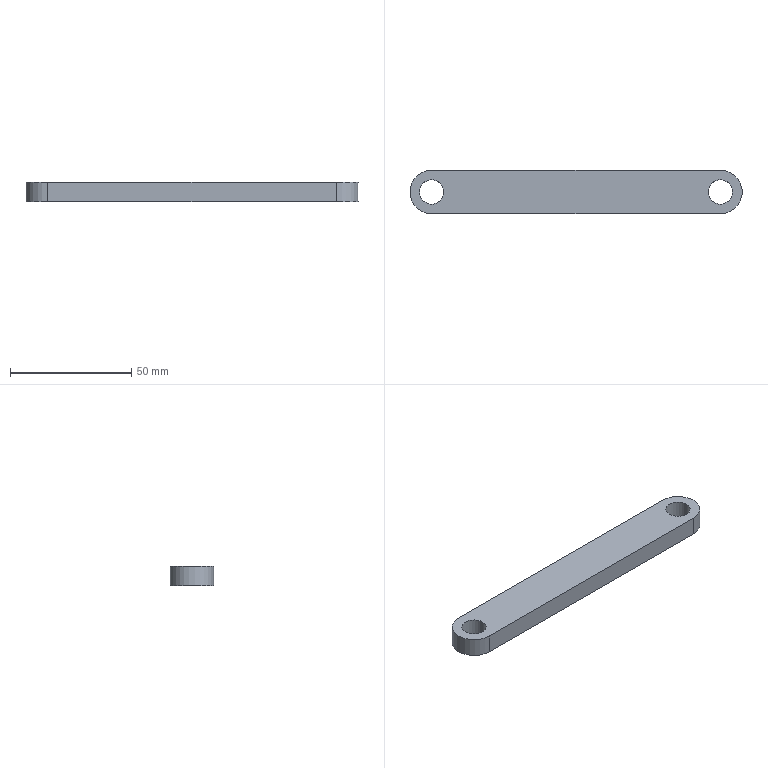Part | STEP file | Crank | 1 solid | 8 faces | box 136.8 x 18 x 8 mm | volume 17886 mm3 | plane 4 | cylinder 4 | commonest cylinder face diameters 10 x2 18 x2
STEP:
#1=CARTESIAN_POINT('',(0.,0.,0.));
#2=DIRECTION('',(0.,0.,1.));
#3=DIRECTION('',(1.,0.,0.));
#4=AXIS2_PLACEMENT_3D('',#1,#2,#3);
#5=CARTESIAN_POINT('',(123.8,0.,8.));
#6=VERTEX_POINT('',#5);
#7=CARTESIAN_POINT('',(118.8,0.,8.));
#8=DIRECTION('',(0.,0.,1.));
#9=DIRECTION('',(1.,0.,0.));
#10=AXIS2_PLACEMENT_3D('',#7,#8,#9);
#11=CIRCLE('',#10,5.);
#12=CARTESIAN_POINT('',(0.,0.,8.));
#13=DIRECTION('',(0.,0.,1.));
#14=DIRECTION('',(1.,0.,0.));
#15=AXIS2_PLACEMENT_3D('',#12,#13,#14);
#16=PLANE('',#15);
#17=CARTESIAN_POINT('',(118.8,0.));
#18=DIRECTION('',(1.,0.));
#19=AXIS2_PLACEMENT_2D('',#17,#18);
#20=CIRCLE('',#19,5.);
#21=(GEOMETRIC_REPRESENTATION_CONTEXT(2)PARAMETRIC_REPRESENTATION_CONTEXT()REPRESENTATION_CONTEXT('',''));
#22=DEFINITIONAL_REPRESENTATION('',(#20),#21);
#23=PCURVE('',#16,#22);
#24=CARTESIAN_POINT('',(118.8,0.,8.));
#25=DIRECTION('',(0.,0.,-1.));
#26=DIRECTION('',(-1.,0.,0.));
#27=AXIS2_PLACEMENT_3D('',#24,#25,#26);
#28=CYLINDRICAL_SURFACE('',#27,5.);
#29=CARTESIAN_POINT('',(9.425,0.));
#30=DIRECTION('',(-1.,0.));
#31=VECTOR('',#30,1.);
#32=LINE('',#29,#31);
#33=(GEOMETRIC_REPRESENTATION_CONTEXT(2)PARAMETRIC_REPRESENTATION_CONTEXT()REPRESENTATION_CONTEXT('',''));
#34=DEFINITIONAL_REPRESENTATION('',(#32),#33);
#35=PCURVE('',#28,#34);
#36=SURFACE_CURVE('',#11,(#23,#35),.PCURVE_S1.);
#37=EDGE_CURVE('',#6,#6,#36,.T.);
#38=ORIENTED_EDGE('',*,*,#37,.F.);
#39=EDGE_LOOP('',(#38));
#40=FACE_BOUND('',#39,.T.);
#41=CARTESIAN_POINT('',(0.,9.,8.));
#42=VERTEX_POINT('',#41);
#43=CARTESIAN_POINT('',(0.,-9.,8.));
#44=VERTEX_POINT('',#43);
#45=CARTESIAN_POINT('',(0.,0.,8.));
#46=DIRECTION('',(0.,0.,1.));
#47=DIRECTION('',(1.,0.,0.));
#48=AXIS2_PLACEMENT_3D('',#45,#46,#47);
#49=CIRCLE('',#48,9.);
#50=CARTESIAN_POINT('',(0.,0.));
#51=DIRECTION('',(1.,0.));
#52=AXIS2_PLACEMENT_2D('',#50,#51);
#53=CIRCLE('',#52,9.);
#54=(GEOMETRIC_REPRESENTATION_CONTEXT(2)PARAMETRIC_REPRESENTATION_CONTEXT()REPRESENTATION_CONTEXT('',''));
#55=DEFINITIONAL_REPRESENTATION('',(#53),#54);
#56=PCURVE('',#16,#55);
#57=CARTESIAN_POINT('',(0.,0.,8.));
#58=DIRECTION('',(0.,0.,-1.));
#59=DIRECTION('',(-1.,0.,0.));
#60=AXIS2_PLACEMENT_3D('',#57,#58,#59);
#61=CYLINDRICAL_SURFACE('',#60,9.);
#62=CARTESIAN_POINT('',(3.142,0.));
#63=DIRECTION('',(-1.,0.));
#64=VECTOR('',#63,1.);
#65=LINE('',#62,#64);
#66=(GEOMETRIC_REPRESENTATION_CONTEXT(2)PARAMETRIC_REPRESENTATION_CONTEXT()REPRESENTATION_CONTEXT('',''));
#67=DEFINITIONAL_REPRESENTATION('',(#65),#66);
#68=PCURVE('',#61,#67);
#69=SURFACE_CURVE('',#49,(#56,#68),.PCURVE_S1.);
#70=EDGE_CURVE('',#42,#44,#69,.T.);
#71=ORIENTED_EDGE('',*,*,#70,.T.);
#72=CARTESIAN_POINT('',(118.8,-9.,8.));
#73=VERTEX_POINT('',#72);
#74=CARTESIAN_POINT('',(0.,-9.,8.));
#75=DIRECTION('',(1.,0.,0.));
#76=VECTOR('',#75,1.);
#77=LINE('',#74,#76);
#78=CARTESIAN_POINT('',(0.,-9.));
#79=DIRECTION('',(1.,0.));
#80=VECTOR('',#79,1.);
#81=LINE('',#78,#80);
#82=(GEOMETRIC_REPRESENTATION_CONTEXT(2)PARAMETRIC_REPRESENTATION_CONTEXT()REPRESENTATION_CONTEXT('',''));
#83=DEFINITIONAL_REPRESENTATION('',(#81),#82);
#84=PCURVE('',#16,#83);
#85=CARTESIAN_POINT('',(0.,-9.,8.));
#86=DIRECTION('',(0.,1.,0.));
#87=DIRECTION('',(0.,0.,1.));
#88=AXIS2_PLACEMENT_3D('',#85,#86,#87);
#89=PLANE('',#88);
#90=CARTESIAN_POINT('',(0.,0.));
#91=DIRECTION('',(0.,1.));
#92=VECTOR('',#91,1.);
#93=LINE('',#90,#92);
#94=(GEOMETRIC_REPRESENTATION_CONTEXT(2)PARAMETRIC_REPRESENTATION_CONTEXT()REPRESENTATION_CONTEXT('',''));
#95=DEFINITIONAL_REPRESENTATION('',(#93),#94);
#96=PCURVE('',#89,#95);
#97=SURFACE_CURVE('',#77,(#84,#96),.PCURVE_S1.);
#98=EDGE_CURVE('',#44,#73,#97,.T.);
#99=ORIENTED_EDGE('',*,*,#98,.T.);
#100=CARTESIAN_POINT('',(118.8,9.,8.));
#101=VERTEX_POINT('',#100);
#102=CARTESIAN_POINT('',(118.8,0.,8.));
#103=DIRECTION('',(0.,0.,1.));
#104=DIRECTION('',(1.,0.,0.));
#105=AXIS2_PLACEMENT_3D('',#102,#103,#104);
#106=CIRCLE('',#105,9.);
#107=CARTESIAN_POINT('',(118.8,0.));
#108=DIRECTION('',(1.,0.));
#109=AXIS2_PLACEMENT_2D('',#107,#108);
#110=CIRCLE('',#109,9.);
#111=(GEOMETRIC_REPRESENTATION_CONTEXT(2)PARAMETRIC_REPRESENTATION_CONTEXT()REPRESENTATION_CONTEXT('',''));
#112=DEFINITIONAL_REPRESENTATION('',(#110),#111);
#113=PCURVE('',#16,#112);
#114=CARTESIAN_POINT('',(118.8,0.,8.));
#115=DIRECTION('',(0.,0.,-1.));
#116=DIRECTION('',(-1.,0.,0.));
#117=AXIS2_PLACEMENT_3D('',#114,#115,#116);
#118=CYLINDRICAL_SURFACE('',#117,9.);
#119=CARTESIAN_POINT('',(9.425,0.));
#120=DIRECTION('',(-1.,0.));
#121=VECTOR('',#120,1.);
#122=LINE('',#119,#121);
#123=(GEOMETRIC_REPRESENTATION_CONTEXT(2)PARAMETRIC_REPRESENTATION_CONTEXT()REPRESENTATION_CONTEXT('',''));
#124=DEFINITIONAL_REPRESENTATION('',(#122),#123);
#125=PCURVE('',#118,#124);
#126=SURFACE_CURVE('',#106,(#113,#125),.PCURVE_S1.);
#127=EDGE_CURVE('',#73,#101,#126,.T.);
#128=ORIENTED_EDGE('',*,*,#127,.T.);
#129=CARTESIAN_POINT('',(0.,9.,8.));
#130=DIRECTION('',(-1.,0.,0.));
#131=VECTOR('',#130,1.);
#132=LINE('',#129,#131);
#133=CARTESIAN_POINT('',(0.,9.));
#134=DIRECTION('',(-1.,0.));
#135=VECTOR('',#134,1.);
#136=LINE('',#133,#135);
#137=(GEOMETRIC_REPRESENTATION_CONTEXT(2)PARAMETRIC_REPRESENTATION_CONTEXT()REPRESENTATION_CONTEXT('',''));
#138=DEFINITIONAL_REPRESENTATION('',(#136),#137);
#139=PCURVE('',#16,#138);
#140=CARTESIAN_POINT('',(0.,9.,8.));
#141=DIRECTION('',(0.,-1.,0.));
#142=DIRECTION('',(0.,0.,-1.));
#143=AXIS2_PLACEMENT_3D('',#140,#141,#142);
#144=PLANE('',#143);
#145=CARTESIAN_POINT('',(0.,0.));
#146=DIRECTION('',(0.,-1.));
#147=VECTOR('',#146,1.);
#148=LINE('',#145,#147);
#149=(GEOMETRIC_REPRESENTATION_CONTEXT(2)PARAMETRIC_REPRESENTATION_CONTEXT()REPRESENTATION_CONTEXT('',''));
#150=DEFINITIONAL_REPRESENTATION('',(#148),#149);
#151=PCURVE('',#144,#150);
#152=SURFACE_CURVE('',#132,(#139,#151),.PCURVE_S1.);
#153=EDGE_CURVE('',#101,#42,#152,.T.);
#154=ORIENTED_EDGE('',*,*,#153,.T.);
#155=EDGE_LOOP('',(#71,#99,#128,#154));
#156=FACE_BOUND('',#155,.T.);
#157=CARTESIAN_POINT('',(5.,0.,8.));
#158=VERTEX_POINT('',#157);
#159=CARTESIAN_POINT('',(0.,0.,8.));
#160=DIRECTION('',(0.,0.,1.));
#161=DIRECTION('',(1.,0.,0.));
#162=AXIS2_PLACEMENT_3D('',#159,#160,#161);
#163=CIRCLE('',#162,5.);
#164=CARTESIAN_POINT('',(0.,0.));
#165=DIRECTION('',(1.,0.));
#166=AXIS2_PLACEMENT_2D('',#164,#165);
#167=CIRCLE('',#166,5.);
#168=(GEOMETRIC_REPRESENTATION_CONTEXT(2)PARAMETRIC_REPRESENTATION_CONTEXT()REPRESENTATION_CONTEXT('',''));
#169=DEFINITIONAL_REPRESENTATION('',(#167),#168);
#170=PCURVE('',#16,#169);
#171=CARTESIAN_POINT('',(0.,0.,8.));
#172=DIRECTION('',(0.,0.,-1.));
#173=DIRECTION('',(-1.,0.,0.));
#174=AXIS2_PLACEMENT_3D('',#171,#172,#173);
#175=CYLINDRICAL_SURFACE('',#174,5.);
#176=CARTESIAN_POINT('',(9.425,0.));
#177=DIRECTION('',(-1.,0.));
#178=VECTOR('',#177,1.);
#179=LINE('',#176,#178);
#180=(GEOMETRIC_REPRESENTATION_CONTEXT(2)PARAMETRIC_REPRESENTATION_CONTEXT()REPRESENTATION_CONTEXT('',''));
#181=DEFINITIONAL_REPRESENTATION('',(#179),#180);
#182=PCURVE('',#175,#181);
#183=SURFACE_CURVE('',#163,(#170,#182),.PCURVE_S1.);
#184=EDGE_CURVE('',#158,#158,#183,.T.);
#185=ORIENTED_EDGE('',*,*,#184,.F.);
#186=EDGE_LOOP('',(#185));
#187=FACE_BOUND('',#186,.T.);
#188=ADVANCED_FACE('',(#40,#156,#187),#16,.T.);
#189=CARTESIAN_POINT('',(0.,9.,0.));
#190=VERTEX_POINT('',#189);
#191=CARTESIAN_POINT('',(0.,-9.,0.));
#192=VERTEX_POINT('',#191);
#193=CARTESIAN_POINT('',(0.,0.,0.));
#194=DIRECTION('',(0.,0.,1.));
#195=DIRECTION('',(1.,0.,0.));
#196=AXIS2_PLACEMENT_3D('',#193,#194,#195);
#197=CIRCLE('',#196,9.);
#198=CARTESIAN_POINT('',(0.,0.,0.));
#199=DIRECTION('',(0.,0.,1.));
#200=DIRECTION('',(1.,0.,0.));
#201=AXIS2_PLACEMENT_3D('',#198,#199,#200);
#202=PLANE('',#201);
#203=CARTESIAN_POINT('',(0.,0.));
#204=DIRECTION('',(1.,0.));
#205=AXIS2_PLACEMENT_2D('',#203,#204);
#206=CIRCLE('',#205,9.);
#207=(GEOMETRIC_REPRESENTATION_CONTEXT(2)PARAMETRIC_REPRESENTATION_CONTEXT()REPRESENTATION_CONTEXT('',''));
#208=DEFINITIONAL_REPRESENTATION('',(#206),#207);
#209=PCURVE('',#202,#208);
#210=CARTESIAN_POINT('',(3.142,8.));
#211=DIRECTION('',(-1.,0.));
#212=VECTOR('',#211,1.);
#213=LINE('',#210,#212);
#214=(GEOMETRIC_REPRESENTATION_CONTEXT(2)PARAMETRIC_REPRESENTATION_CONTEXT()REPRESENTATION_CONTEXT('',''));
#215=DEFINITIONAL_REPRESENTATION('',(#213),#214);
#216=PCURVE('',#61,#215);
#217=SURFACE_CURVE('',#197,(#209,#216),.PCURVE_S1.);
#218=EDGE_CURVE('',#190,#192,#217,.T.);
#219=ORIENTED_EDGE('',*,*,#218,.F.);
#220=CARTESIAN_POINT('',(118.8,9.,0.));
#221=VERTEX_POINT('',#220);
#222=CARTESIAN_POINT('',(0.,9.,0.));
#223=DIRECTION('',(-1.,0.,0.));
#224=VECTOR('',#223,1.);
#225=LINE('',#222,#224);
#226=CARTESIAN_POINT('',(0.,9.));
#227=DIRECTION('',(-1.,0.));
#228=VECTOR('',#227,1.);
#229=LINE('',#226,#228);
#230=(GEOMETRIC_REPRESENTATION_CONTEXT(2)PARAMETRIC_REPRESENTATION_CONTEXT()REPRESENTATION_CONTEXT('',''));
#231=DEFINITIONAL_REPRESENTATION('',(#229),#230);
#232=PCURVE('',#202,#231);
#233=CARTESIAN_POINT('',(8.,0.));
#234=DIRECTION('',(0.,-1.));
#235=VECTOR('',#234,1.);
#236=LINE('',#233,#235);
#237=(GEOMETRIC_REPRESENTATION_CONTEXT(2)PARAMETRIC_REPRESENTATION_CONTEXT()REPRESENTATION_CONTEXT('',''));
#238=DEFINITIONAL_REPRESENTATION('',(#236),#237);
#239=PCURVE('',#144,#238);
#240=SURFACE_CURVE('',#225,(#232,#239),.PCURVE_S1.);
#241=EDGE_CURVE('',#221,#190,#240,.T.);
#242=ORIENTED_EDGE('',*,*,#241,.F.);
#243=CARTESIAN_POINT('',(118.8,-9.,0.));
#244=VERTEX_POINT('',#243);
#245=CARTESIAN_POINT('',(118.8,0.,0.));
#246=DIRECTION('',(0.,0.,1.));
#247=DIRECTION('',(1.,0.,0.));
#248=AXIS2_PLACEMENT_3D('',#245,#246,#247);
#249=CIRCLE('',#248,9.);
#250=CARTESIAN_POINT('',(118.8,0.));
#251=DIRECTION('',(1.,0.));
#252=AXIS2_PLACEMENT_2D('',#250,#251);
#253=CIRCLE('',#252,9.);
#254=(GEOMETRIC_REPRESENTATION_CONTEXT(2)PARAMETRIC_REPRESENTATION_CONTEXT()REPRESENTATION_CONTEXT('',''));
#255=DEFINITIONAL_REPRESENTATION('',(#253),#254);
#256=PCURVE('',#202,#255);
#257=CARTESIAN_POINT('',(9.425,8.));
#258=DIRECTION('',(-1.,0.));
#259=VECTOR('',#258,1.);
#260=LINE('',#257,#259);
#261=(GEOMETRIC_REPRESENTATION_CONTEXT(2)PARAMETRIC_REPRESENTATION_CONTEXT()REPRESENTATION_CONTEXT('',''));
#262=DEFINITIONAL_REPRESENTATION('',(#260),#261);
#263=PCURVE('',#118,#262);
#264=SURFACE_CURVE('',#249,(#256,#263),.PCURVE_S1.);
#265=EDGE_CURVE('',#244,#221,#264,.T.);
#266=ORIENTED_EDGE('',*,*,#265,.F.);
#267=CARTESIAN_POINT('',(0.,-9.,0.));
#268=DIRECTION('',(1.,0.,0.));
#269=VECTOR('',#268,1.);
#270=LINE('',#267,#269);
#271=CARTESIAN_POINT('',(0.,-9.));
#272=DIRECTION('',(1.,0.));
#273=VECTOR('',#272,1.);
#274=LINE('',#271,#273);
#275=(GEOMETRIC_REPRESENTATION_CONTEXT(2)PARAMETRIC_REPRESENTATION_CONTEXT()REPRESENTATION_CONTEXT('',''));
#276=DEFINITIONAL_REPRESENTATION('',(#274),#275);
#277=PCURVE('',#202,#276);
#278=CARTESIAN_POINT('',(-8.,0.));
#279=DIRECTION('',(0.,1.));
#280=VECTOR('',#279,1.);
#281=LINE('',#278,#280);
#282=(GEOMETRIC_REPRESENTATION_CONTEXT(2)PARAMETRIC_REPRESENTATION_CONTEXT()REPRESENTATION_CONTEXT('',''));
#283=DEFINITIONAL_REPRESENTATION('',(#281),#282);
#284=PCURVE('',#89,#283);
#285=SURFACE_CURVE('',#270,(#277,#284),.PCURVE_S1.);
#286=EDGE_CURVE('',#192,#244,#285,.T.);
#287=ORIENTED_EDGE('',*,*,#286,.F.);
#288=EDGE_LOOP('',(#219,#242,#266,#287));
#289=FACE_BOUND('',#288,.T.);
#290=CARTESIAN_POINT('',(123.8,0.,0.));
#291=VERTEX_POINT('',#290);
#292=CARTESIAN_POINT('',(118.8,0.,0.));
#293=DIRECTION('',(0.,0.,1.));
#294=DIRECTION('',(1.,0.,0.));
#295=AXIS2_PLACEMENT_3D('',#292,#293,#294);
#296=CIRCLE('',#295,5.);
#297=CARTESIAN_POINT('',(118.8,0.));
#298=DIRECTION('',(1.,0.));
#299=AXIS2_PLACEMENT_2D('',#297,#298);
#300=CIRCLE('',#299,5.);
#301=(GEOMETRIC_REPRESENTATION_CONTEXT(2)PARAMETRIC_REPRESENTATION_CONTEXT()REPRESENTATION_CONTEXT('',''));
#302=DEFINITIONAL_REPRESENTATION('',(#300),#301);
#303=PCURVE('',#202,#302);
#304=CARTESIAN_POINT('',(9.425,8.));
#305=DIRECTION('',(-1.,0.));
#306=VECTOR('',#305,1.);
#307=LINE('',#304,#306);
#308=(GEOMETRIC_REPRESENTATION_CONTEXT(2)PARAMETRIC_REPRESENTATION_CONTEXT()REPRESENTATION_CONTEXT('',''));
#309=DEFINITIONAL_REPRESENTATION('',(#307),#308);
#310=PCURVE('',#28,#309);
#311=SURFACE_CURVE('',#296,(#303,#310),.PCURVE_S1.);
#312=EDGE_CURVE('',#291,#291,#311,.T.);
#313=ORIENTED_EDGE('',*,*,#312,.T.);
#314=EDGE_LOOP('',(#313));
#315=FACE_BOUND('',#314,.T.);
#316=CARTESIAN_POINT('',(5.,0.,0.));
#317=VERTEX_POINT('',#316);
#318=CARTESIAN_POINT('',(0.,0.,0.));
#319=DIRECTION('',(0.,0.,1.));
#320=DIRECTION('',(1.,0.,0.));
#321=AXIS2_PLACEMENT_3D('',#318,#319,#320);
#322=CIRCLE('',#321,5.);
#323=CARTESIAN_POINT('',(0.,0.));
#324=DIRECTION('',(1.,0.));
#325=AXIS2_PLACEMENT_2D('',#323,#324);
#326=CIRCLE('',#325,5.);
#327=(GEOMETRIC_REPRESENTATION_CONTEXT(2)PARAMETRIC_REPRESENTATION_CONTEXT()REPRESENTATION_CONTEXT('',''));
#328=DEFINITIONAL_REPRESENTATION('',(#326),#327);
#329=PCURVE('',#202,#328);
#330=CARTESIAN_POINT('',(9.425,8.));
#331=DIRECTION('',(-1.,0.));
#332=VECTOR('',#331,1.);
#333=LINE('',#330,#332);
#334=(GEOMETRIC_REPRESENTATION_CONTEXT(2)PARAMETRIC_REPRESENTATION_CONTEXT()REPRESENTATION_CONTEXT('',''));
#335=DEFINITIONAL_REPRESENTATION('',(#333),#334);
#336=PCURVE('',#175,#335);
#337=SURFACE_CURVE('',#322,(#329,#336),.PCURVE_S1.);
#338=EDGE_CURVE('',#317,#317,#337,.T.);
#339=ORIENTED_EDGE('',*,*,#338,.T.);
#340=EDGE_LOOP('',(#339));
#341=FACE_BOUND('',#340,.T.);
#342=ADVANCED_FACE('',(#289,#315,#341),#202,.F.);
#343=ORIENTED_EDGE('',*,*,#218,.T.);
#344=CARTESIAN_POINT('',(0.,-9.,8.));
#345=DIRECTION('',(0.,0.,-1.));
#346=VECTOR('',#345,1.);
#347=LINE('',#344,#346);
#348=CARTESIAN_POINT('',(-1.571,0.));
#349=DIRECTION('',(0.,1.));
#350=VECTOR('',#349,1.);
#351=LINE('',#348,#350);
#352=(GEOMETRIC_REPRESENTATION_CONTEXT(2)PARAMETRIC_REPRESENTATION_CONTEXT()REPRESENTATION_CONTEXT('',''));
#353=DEFINITIONAL_REPRESENTATION('',(#351),#352);
#354=PCURVE('',#61,#353);
#355=CARTESIAN_POINT('',(0.,0.));
#356=DIRECTION('',(-1.,0.));
#357=VECTOR('',#356,1.);
#358=LINE('',#355,#357);
#359=(GEOMETRIC_REPRESENTATION_CONTEXT(2)PARAMETRIC_REPRESENTATION_CONTEXT()REPRESENTATION_CONTEXT('',''));
#360=DEFINITIONAL_REPRESENTATION('',(#358),#359);
#361=PCURVE('',#89,#360);
#362=SURFACE_CURVE('',#347,(#354,#361),.PCURVE_S1.);
#363=EDGE_CURVE('',#44,#192,#362,.T.);
#364=ORIENTED_EDGE('',*,*,#363,.F.);
#365=ORIENTED_EDGE('',*,*,#70,.F.);
#366=CARTESIAN_POINT('',(0.,9.,8.));
#367=DIRECTION('',(0.,0.,-1.));
#368=VECTOR('',#367,1.);
#369=LINE('',#366,#368);
#370=CARTESIAN_POINT('',(1.571,0.));
#371=DIRECTION('',(0.,1.));
#372=VECTOR('',#371,1.);
#373=LINE('',#370,#372);
#374=(GEOMETRIC_REPRESENTATION_CONTEXT(2)PARAMETRIC_REPRESENTATION_CONTEXT()REPRESENTATION_CONTEXT('',''));
#375=DEFINITIONAL_REPRESENTATION('',(#373),#374);
#376=PCURVE('',#61,#375);
#377=CARTESIAN_POINT('',(0.,0.));
#378=DIRECTION('',(1.,0.));
#379=VECTOR('',#378,1.);
#380=LINE('',#377,#379);
#381=(GEOMETRIC_REPRESENTATION_CONTEXT(2)PARAMETRIC_REPRESENTATION_CONTEXT()REPRESENTATION_CONTEXT('',''));
#382=DEFINITIONAL_REPRESENTATION('',(#380),#381);
#383=PCURVE('',#144,#382);
#384=SURFACE_CURVE('',#369,(#376,#383),.PCURVE_S1.);
#385=EDGE_CURVE('',#42,#190,#384,.T.);
#386=ORIENTED_EDGE('',*,*,#385,.T.);
#387=EDGE_LOOP('',(#343,#364,#365,#386));
#388=FACE_BOUND('',#387,.T.);
#389=ADVANCED_FACE('',(#388),#61,.T.);
#390=ORIENTED_EDGE('',*,*,#286,.T.);
#391=CARTESIAN_POINT('',(118.8,-9.,8.));
#392=DIRECTION('',(0.,0.,-1.));
#393=VECTOR('',#392,1.);
#394=LINE('',#391,#393);
#395=CARTESIAN_POINT('',(0.,118.8));
#396=DIRECTION('',(-1.,0.));
#397=VECTOR('',#396,1.);
#398=LINE('',#395,#397);
#399=(GEOMETRIC_REPRESENTATION_CONTEXT(2)PARAMETRIC_REPRESENTATION_CONTEXT()REPRESENTATION_CONTEXT('',''));
#400=DEFINITIONAL_REPRESENTATION('',(#398),#399);
#401=PCURVE('',#89,#400);
#402=CARTESIAN_POINT('',(4.712,0.));
#403=DIRECTION('',(0.,1.));
#404=VECTOR('',#403,1.);
#405=LINE('',#402,#404);
#406=(GEOMETRIC_REPRESENTATION_CONTEXT(2)PARAMETRIC_REPRESENTATION_CONTEXT()REPRESENTATION_CONTEXT('',''));
#407=DEFINITIONAL_REPRESENTATION('',(#405),#406);
#408=PCURVE('',#118,#407);
#409=SURFACE_CURVE('',#394,(#401,#408),.PCURVE_S1.);
#410=EDGE_CURVE('',#73,#244,#409,.T.);
#411=ORIENTED_EDGE('',*,*,#410,.F.);
#412=ORIENTED_EDGE('',*,*,#98,.F.);
#413=ORIENTED_EDGE('',*,*,#363,.T.);
#414=EDGE_LOOP('',(#390,#411,#412,#413));
#415=FACE_BOUND('',#414,.T.);
#416=ADVANCED_FACE('',(#415),#89,.F.);
#417=ORIENTED_EDGE('',*,*,#265,.T.);
#418=CARTESIAN_POINT('',(118.8,9.,8.));
#419=DIRECTION('',(0.,0.,-1.));
#420=VECTOR('',#419,1.);
#421=LINE('',#418,#420);
#422=CARTESIAN_POINT('',(1.571,0.));
#423=DIRECTION('',(0.,1.));
#424=VECTOR('',#423,1.);
#425=LINE('',#422,#424);
#426=(GEOMETRIC_REPRESENTATION_CONTEXT(2)PARAMETRIC_REPRESENTATION_CONTEXT()REPRESENTATION_CONTEXT('',''));
#427=DEFINITIONAL_REPRESENTATION('',(#425),#426);
#428=PCURVE('',#118,#427);
#429=CARTESIAN_POINT('',(0.,118.8));
#430=DIRECTION('',(1.,0.));
#431=VECTOR('',#430,1.);
#432=LINE('',#429,#431);
#433=(GEOMETRIC_REPRESENTATION_CONTEXT(2)PARAMETRIC_REPRESENTATION_CONTEXT()REPRESENTATION_CONTEXT('',''));
#434=DEFINITIONAL_REPRESENTATION('',(#432),#433);
#435=PCURVE('',#144,#434);
#436=SURFACE_CURVE('',#421,(#428,#435),.PCURVE_S1.);
#437=EDGE_CURVE('',#101,#221,#436,.T.);
#438=ORIENTED_EDGE('',*,*,#437,.F.);
#439=ORIENTED_EDGE('',*,*,#127,.F.);
#440=ORIENTED_EDGE('',*,*,#410,.T.);
#441=EDGE_LOOP('',(#417,#438,#439,#440));
#442=FACE_BOUND('',#441,.T.);
#443=ADVANCED_FACE('',(#442),#118,.T.);
#444=ORIENTED_EDGE('',*,*,#241,.T.);
#445=ORIENTED_EDGE('',*,*,#385,.F.);
#446=ORIENTED_EDGE('',*,*,#153,.F.);
#447=ORIENTED_EDGE('',*,*,#437,.T.);
#448=EDGE_LOOP('',(#444,#445,#446,#447));
#449=FACE_BOUND('',#448,.T.);
#450=ADVANCED_FACE('',(#449),#144,.F.);
#451=ORIENTED_EDGE('',*,*,#37,.F.);
#452=CARTESIAN_POINT('',(123.8,0.,8.));
#453=CARTESIAN_POINT('',(123.8,0.,0.));
#454=B_SPLINE_CURVE_WITH_KNOTS('',1,(#452,#453),.UNSPECIFIED.,.F.,.F.,(2,2),(0.,8.),.PIECEWISE_BEZIER_KNOTS.);
#455=CARTESIAN_POINT('',(9.425,0.));
#456=DIRECTION('',(0.,1.));
#457=VECTOR('',#456,1.);
#458=LINE('',#455,#457);
#459=(GEOMETRIC_REPRESENTATION_CONTEXT(2)PARAMETRIC_REPRESENTATION_CONTEXT()REPRESENTATION_CONTEXT('',''));
#460=DEFINITIONAL_REPRESENTATION('',(#458),#459);
#461=PCURVE('',#28,#460);
#462=CARTESIAN_POINT('',(3.142,0.));
#463=DIRECTION('',(0.,1.));
#464=VECTOR('',#463,1.);
#465=LINE('',#462,#464);
#466=(GEOMETRIC_REPRESENTATION_CONTEXT(2)PARAMETRIC_REPRESENTATION_CONTEXT()REPRESENTATION_CONTEXT('',''));
#467=DEFINITIONAL_REPRESENTATION('',(#465),#466);
#468=PCURVE('',#28,#467);
#469=SEAM_CURVE('',#454,(#461,#468),.PCURVE_S1.);
#470=EDGE_CURVE('',#6,#291,#469,.T.);
#471=ORIENTED_EDGE('',*,*,#470,.T.);
#472=ORIENTED_EDGE('',*,*,#312,.T.);
#473=ORIENTED_EDGE('',*,*,#470,.F.);
#474=EDGE_LOOP('',(#451,#471,#472,#473));
#475=FACE_BOUND('',#474,.F.);
#476=ADVANCED_FACE('',(#475),#28,.F.);
#477=ORIENTED_EDGE('',*,*,#184,.F.);
#478=CARTESIAN_POINT('',(5.,0.,8.));
#479=CARTESIAN_POINT('',(5.,0.,0.));
#480=B_SPLINE_CURVE_WITH_KNOTS('',1,(#478,#479),.UNSPECIFIED.,.F.,.F.,(2,2),(0.,8.),.PIECEWISE_BEZIER_KNOTS.);
#481=CARTESIAN_POINT('',(9.425,0.));
#482=DIRECTION('',(0.,1.));
#483=VECTOR('',#482,1.);
#484=LINE('',#481,#483);
#485=(GEOMETRIC_REPRESENTATION_CONTEXT(2)PARAMETRIC_REPRESENTATION_CONTEXT()REPRESENTATION_CONTEXT('',''));
#486=DEFINITIONAL_REPRESENTATION('',(#484),#485);
#487=PCURVE('',#175,#486);
#488=CARTESIAN_POINT('',(3.142,0.));
#489=DIRECTION('',(0.,1.));
#490=VECTOR('',#489,1.);
#491=LINE('',#488,#490);
#492=(GEOMETRIC_REPRESENTATION_CONTEXT(2)PARAMETRIC_REPRESENTATION_CONTEXT()REPRESENTATION_CONTEXT('',''));
#493=DEFINITIONAL_REPRESENTATION('',(#491),#492);
#494=PCURVE('',#175,#493);
#495=SEAM_CURVE('',#480,(#487,#494),.PCURVE_S1.);
#496=EDGE_CURVE('',#158,#317,#495,.T.);
#497=ORIENTED_EDGE('',*,*,#496,.T.);
#498=ORIENTED_EDGE('',*,*,#338,.T.);
#499=ORIENTED_EDGE('',*,*,#496,.F.);
#500=EDGE_LOOP('',(#477,#497,#498,#499));
#501=FACE_BOUND('',#500,.F.);
#502=ADVANCED_FACE('',(#501),#175,.F.);
#503=CLOSED_SHELL('',(#188,#342,#389,#416,#443,#450,#476,#502));
#504=MANIFOLD_SOLID_BREP('',#503);
#505=(LENGTH_UNIT()NAMED_UNIT(*)SI_UNIT(.MILLI.,.METRE.));
#506=UNCERTAINTY_MEASURE_WITH_UNIT(LENGTH_MEASURE(0.000002),#505,'','');
#507=(NAMED_UNIT(*)PLANE_ANGLE_UNIT()SI_UNIT($,.RADIAN.));
#508=(NAMED_UNIT(*)SI_UNIT($,.STERADIAN.)SOLID_ANGLE_UNIT());
#509=(GEOMETRIC_REPRESENTATION_CONTEXT(3)GLOBAL_UNCERTAINTY_ASSIGNED_CONTEXT((#506))GLOBAL_UNIT_ASSIGNED_CONTEXT((#505,#507,#508))REPRESENTATION_CONTEXT('',''));
#510=ADVANCED_BREP_SHAPE_REPRESENTATION('',(#4,#504),#509);